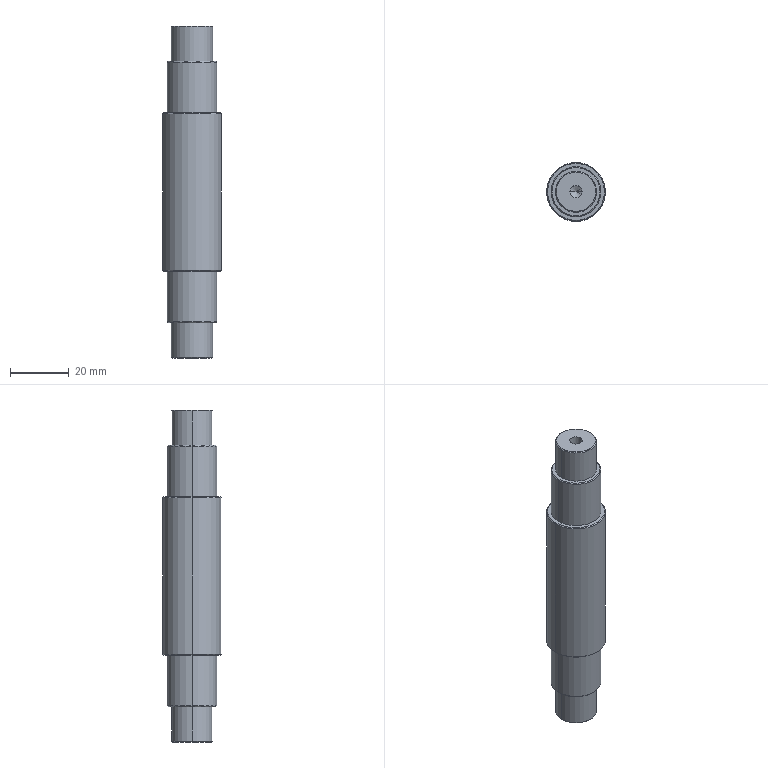Part | NX | features BREP 1 | 1 solid | 36 faces | box 20 x 20 x 113 mm | volume 28190 mm3 | cone 16 | cylinder 14 | plane 6 | commonest cylinder face diameters 4.2 x4 14 x4 17 x4 20 x2
STEP:
#1=CARTESIAN_POINT('',(6.7,0.,56.5));
#2=VERTEX_POINT('',#1);
#3=CARTESIAN_POINT('',(-6.7,0.,56.5));
#4=VERTEX_POINT('',#3);
#5=CARTESIAN_POINT('',(0.,0.,56.5));
#6=DIRECTION('',(0.,0.,1.));
#7=DIRECTION('',(1.,0.,0.));
#8=AXIS2_PLACEMENT_3D('',#5,#6,#7);
#9=CIRCLE('',#8,6.7);
#10=EDGE_CURVE('',#2,#4,#9,.T.);
#11=ORIENTED_EDGE('',*,*,#10,.F.);
#12=CARTESIAN_POINT('',(7.,0.,56.2));
#13=VERTEX_POINT('',#12);
#14=CARTESIAN_POINT('',(6.7,0.,56.5));
#15=DIRECTION('',(0.7071,0.,-0.7071));
#16=VECTOR('',#15,1000.);
#17=LINE('',#14,#16);
#18=EDGE_CURVE('',#2,#13,#17,.T.);
#19=ORIENTED_EDGE('',*,*,#18,.T.);
#20=CARTESIAN_POINT('',(-7.,0.,56.2));
#21=VERTEX_POINT('',#20);
#22=CARTESIAN_POINT('',(0.,0.,56.2));
#23=DIRECTION('',(0.,0.,-1.));
#24=DIRECTION('',(1.,0.,0.));
#25=AXIS2_PLACEMENT_3D('',#22,#23,#24);
#26=CIRCLE('',#25,7.);
#27=EDGE_CURVE('',#21,#13,#26,.T.);
#28=ORIENTED_EDGE('',*,*,#27,.F.);
#29=CARTESIAN_POINT('',(-6.7,0.,56.5));
#30=DIRECTION('',(-0.7071,0.,-0.7071));
#31=VECTOR('',#30,1000.);
#32=LINE('',#29,#31);
#33=EDGE_CURVE('',#4,#21,#32,.T.);
#34=ORIENTED_EDGE('',*,*,#33,.F.);
#35=EDGE_LOOP('',(#11,#19,#28,#34));
#36=FACE_BOUND('',#35,.T.);
#37=CARTESIAN_POINT('',(0.,0.,56.5));
#38=DIRECTION('',(0.,0.,-1.));
#39=DIRECTION('',(-1.,0.,0.));
#40=AXIS2_PLACEMENT_3D('',#37,#38,#39);
#41=CONICAL_SURFACE('',#40,6.7,0.7854);
#42=ADVANCED_FACE('',(#36),#41,.T.);
#43=CARTESIAN_POINT('',(8.2,0.,44.5));
#44=VERTEX_POINT('',#43);
#45=CARTESIAN_POINT('',(-8.2,0.,44.5));
#46=VERTEX_POINT('',#45);
#47=CARTESIAN_POINT('',(0.,0.,44.5));
#48=DIRECTION('',(0.,0.,1.));
#49=DIRECTION('',(1.,0.,0.));
#50=AXIS2_PLACEMENT_3D('',#47,#48,#49);
#51=CIRCLE('',#50,8.2);
#52=EDGE_CURVE('',#44,#46,#51,.T.);
#53=ORIENTED_EDGE('',*,*,#52,.F.);
#54=CARTESIAN_POINT('',(8.5,0.,44.2));
#55=VERTEX_POINT('',#54);
#56=CARTESIAN_POINT('',(8.2,0.,44.5));
#57=DIRECTION('',(0.7071,0.,-0.7071));
#58=VECTOR('',#57,1000.);
#59=LINE('',#56,#58);
#60=EDGE_CURVE('',#44,#55,#59,.T.);
#61=ORIENTED_EDGE('',*,*,#60,.T.);
#62=CARTESIAN_POINT('',(-8.5,0.,44.2));
#63=VERTEX_POINT('',#62);
#64=CARTESIAN_POINT('',(0.,0.,44.2));
#65=DIRECTION('',(0.,0.,-1.));
#66=DIRECTION('',(1.,0.,0.));
#67=AXIS2_PLACEMENT_3D('',#64,#65,#66);
#68=CIRCLE('',#67,8.5);
#69=EDGE_CURVE('',#63,#55,#68,.T.);
#70=ORIENTED_EDGE('',*,*,#69,.F.);
#71=CARTESIAN_POINT('',(-8.2,0.,44.5));
#72=DIRECTION('',(-0.7071,0.,-0.7071));
#73=VECTOR('',#72,1000.);
#74=LINE('',#71,#73);
#75=EDGE_CURVE('',#46,#63,#74,.T.);
#76=ORIENTED_EDGE('',*,*,#75,.F.);
#77=EDGE_LOOP('',(#53,#61,#70,#76));
#78=FACE_BOUND('',#77,.T.);
#79=CARTESIAN_POINT('',(0.,0.,44.5));
#80=DIRECTION('',(0.,0.,-1.));
#81=DIRECTION('',(-1.,0.,0.));
#82=AXIS2_PLACEMENT_3D('',#79,#80,#81);
#83=CONICAL_SURFACE('',#82,8.2,0.7854);
#84=ADVANCED_FACE('',(#78),#83,.T.);
#85=CARTESIAN_POINT('',(9.7,0.,27.));
#86=VERTEX_POINT('',#85);
#87=CARTESIAN_POINT('',(-9.7,0.,27.));
#88=VERTEX_POINT('',#87);
#89=CARTESIAN_POINT('',(0.,0.,27.));
#90=DIRECTION('',(0.,0.,1.));
#91=DIRECTION('',(1.,0.,0.));
#92=AXIS2_PLACEMENT_3D('',#89,#90,#91);
#93=CIRCLE('',#92,9.7);
#94=EDGE_CURVE('',#86,#88,#93,.T.);
#95=ORIENTED_EDGE('',*,*,#94,.F.);
#96=CARTESIAN_POINT('',(10.,0.,26.7));
#97=VERTEX_POINT('',#96);
#98=CARTESIAN_POINT('',(10.,0.,26.7));
#99=DIRECTION('',(0.7071,0.,-0.7071));
#100=VECTOR('',#99,1000.);
#101=LINE('',#98,#100);
#102=EDGE_CURVE('',#86,#97,#101,.T.);
#103=ORIENTED_EDGE('',*,*,#102,.T.);
#104=CARTESIAN_POINT('',(-10.,0.,26.7));
#105=VERTEX_POINT('',#104);
#106=CARTESIAN_POINT('',(0.,0.,26.7));
#107=DIRECTION('',(0.,0.,-1.));
#108=DIRECTION('',(1.,0.,0.));
#109=AXIS2_PLACEMENT_3D('',#106,#107,#108);
#110=CIRCLE('',#109,10.);
#111=EDGE_CURVE('',#105,#97,#110,.T.);
#112=ORIENTED_EDGE('',*,*,#111,.F.);
#113=CARTESIAN_POINT('',(-10.,0.,26.7));
#114=DIRECTION('',(-0.7071,0.,-0.7071));
#115=VECTOR('',#114,1000.);
#116=LINE('',#113,#115);
#117=EDGE_CURVE('',#88,#105,#116,.T.);
#118=ORIENTED_EDGE('',*,*,#117,.F.);
#119=EDGE_LOOP('',(#95,#103,#112,#118));
#120=FACE_BOUND('',#119,.T.);
#121=CARTESIAN_POINT('',(0.,0.,26.7));
#122=DIRECTION('',(0.,0.,-1.));
#123=DIRECTION('',(-1.,0.,0.));
#124=AXIS2_PLACEMENT_3D('',#121,#122,#123);
#125=CONICAL_SURFACE('',#124,10.,0.7854);
#126=ADVANCED_FACE('',(#120),#125,.T.);
#127=CARTESIAN_POINT('',(-9.7,0.,-27.));
#128=VERTEX_POINT('',#127);
#129=CARTESIAN_POINT('',(9.7,0.,-27.));
#130=VERTEX_POINT('',#129);
#131=CARTESIAN_POINT('',(0.,0.,-27.));
#132=DIRECTION('',(0.,0.,-1.));
#133=DIRECTION('',(-1.,0.,0.));
#134=AXIS2_PLACEMENT_3D('',#131,#132,#133);
#135=CIRCLE('',#134,9.7);
#136=EDGE_CURVE('',#128,#130,#135,.T.);
#137=ORIENTED_EDGE('',*,*,#136,.F.);
#138=CARTESIAN_POINT('',(-10.,0.,-26.7));
#139=VERTEX_POINT('',#138);
#140=CARTESIAN_POINT('',(-9.7,0.,-27.));
#141=DIRECTION('',(-0.7071,0.,0.7071));
#142=VECTOR('',#141,1000.);
#143=LINE('',#140,#142);
#144=EDGE_CURVE('',#139,#128,#143,.F.);
#145=ORIENTED_EDGE('',*,*,#144,.F.);
#146=CARTESIAN_POINT('',(10.,0.,-26.7));
#147=VERTEX_POINT('',#146);
#148=CARTESIAN_POINT('',(0.,0.,-26.7));
#149=DIRECTION('',(0.,0.,1.));
#150=DIRECTION('',(-1.,0.,0.));
#151=AXIS2_PLACEMENT_3D('',#148,#149,#150);
#152=CIRCLE('',#151,10.);
#153=EDGE_CURVE('',#147,#139,#152,.T.);
#154=ORIENTED_EDGE('',*,*,#153,.F.);
#155=CARTESIAN_POINT('',(9.7,0.,-27.));
#156=DIRECTION('',(0.7071,0.,0.7071));
#157=VECTOR('',#156,1000.);
#158=LINE('',#155,#157);
#159=EDGE_CURVE('',#147,#130,#158,.F.);
#160=ORIENTED_EDGE('',*,*,#159,.T.);
#161=EDGE_LOOP('',(#137,#145,#154,#160));
#162=FACE_BOUND('',#161,.T.);
#163=CARTESIAN_POINT('',(0.,0.,-27.));
#164=DIRECTION('',(0.,0.,1.));
#165=DIRECTION('',(1.,0.,0.));
#166=AXIS2_PLACEMENT_3D('',#163,#164,#165);
#167=CONICAL_SURFACE('',#166,9.7,0.7854);
#168=ADVANCED_FACE('',(#162),#167,.T.);
#169=CARTESIAN_POINT('',(-8.2,0.,-44.5));
#170=VERTEX_POINT('',#169);
#171=CARTESIAN_POINT('',(8.2,0.,-44.5));
#172=VERTEX_POINT('',#171);
#173=CARTESIAN_POINT('',(0.,0.,-44.5));
#174=DIRECTION('',(0.,0.,-1.));
#175=DIRECTION('',(1.,0.,0.));
#176=AXIS2_PLACEMENT_3D('',#173,#174,#175);
#177=CIRCLE('',#176,8.2);
#178=EDGE_CURVE('',#170,#172,#177,.T.);
#179=ORIENTED_EDGE('',*,*,#178,.F.);
#180=CARTESIAN_POINT('',(-8.5,0.,-44.2));
#181=VERTEX_POINT('',#180);
#182=CARTESIAN_POINT('',(-8.5,0.,-44.2));
#183=DIRECTION('',(-0.7071,0.,0.7071));
#184=VECTOR('',#183,1000.);
#185=LINE('',#182,#184);
#186=EDGE_CURVE('',#181,#170,#185,.F.);
#187=ORIENTED_EDGE('',*,*,#186,.F.);
#188=CARTESIAN_POINT('',(8.5,0.,-44.2));
#189=VERTEX_POINT('',#188);
#190=CARTESIAN_POINT('',(0.,0.,-44.2));
#191=DIRECTION('',(0.,0.,1.));
#192=DIRECTION('',(1.,0.,0.));
#193=AXIS2_PLACEMENT_3D('',#190,#191,#192);
#194=CIRCLE('',#193,8.5);
#195=EDGE_CURVE('',#189,#181,#194,.T.);
#196=ORIENTED_EDGE('',*,*,#195,.F.);
#197=CARTESIAN_POINT('',(8.5,0.,-44.2));
#198=DIRECTION('',(0.7071,0.,0.7071));
#199=VECTOR('',#198,1000.);
#200=LINE('',#197,#199);
#201=EDGE_CURVE('',#189,#172,#200,.F.);
#202=ORIENTED_EDGE('',*,*,#201,.T.);
#203=EDGE_LOOP('',(#179,#187,#196,#202));
#204=FACE_BOUND('',#203,.T.);
#205=CARTESIAN_POINT('',(0.,0.,-44.2));
#206=DIRECTION('',(0.,0.,1.));
#207=DIRECTION('',(1.,0.,0.));
#208=AXIS2_PLACEMENT_3D('',#205,#206,#207);
#209=CONICAL_SURFACE('',#208,8.5,0.7854);
#210=ADVANCED_FACE('',(#204),#209,.T.);
#211=CARTESIAN_POINT('',(-6.7,0.,-56.5));
#212=VERTEX_POINT('',#211);
#213=CARTESIAN_POINT('',(6.7,0.,-56.5));
#214=VERTEX_POINT('',#213);
#215=CARTESIAN_POINT('',(0.,0.,-56.5));
#216=DIRECTION('',(0.,0.,-1.));
#217=DIRECTION('',(-1.,0.,0.));
#218=AXIS2_PLACEMENT_3D('',#215,#216,#217);
#219=CIRCLE('',#218,6.7);
#220=EDGE_CURVE('',#212,#214,#219,.T.);
#221=ORIENTED_EDGE('',*,*,#220,.F.);
#222=CARTESIAN_POINT('',(-7.,0.,-56.2));
#223=VERTEX_POINT('',#222);
#224=CARTESIAN_POINT('',(-6.7,0.,-56.5));
#225=DIRECTION('',(-0.7071,0.,0.7071));
#226=VECTOR('',#225,1000.);
#227=LINE('',#224,#226);
#228=EDGE_CURVE('',#223,#212,#227,.F.);
#229=ORIENTED_EDGE('',*,*,#228,.F.);
#230=CARTESIAN_POINT('',(7.,0.,-56.2));
#231=VERTEX_POINT('',#230);
#232=CARTESIAN_POINT('',(0.,0.,-56.2));
#233=DIRECTION('',(0.,0.,1.));
#234=DIRECTION('',(-1.,0.,0.));
#235=AXIS2_PLACEMENT_3D('',#232,#233,#234);
#236=CIRCLE('',#235,7.);
#237=EDGE_CURVE('',#231,#223,#236,.T.);
#238=ORIENTED_EDGE('',*,*,#237,.F.);
#239=CARTESIAN_POINT('',(6.7,0.,-56.5));
#240=DIRECTION('',(0.7071,0.,0.7071));
#241=VECTOR('',#240,1000.);
#242=LINE('',#239,#241);
#243=EDGE_CURVE('',#231,#214,#242,.F.);
#244=ORIENTED_EDGE('',*,*,#243,.T.);
#245=EDGE_LOOP('',(#221,#229,#238,#244));
#246=FACE_BOUND('',#245,.T.);
#247=CARTESIAN_POINT('',(0.,0.,-56.5));
#248=DIRECTION('',(0.,0.,1.));
#249=DIRECTION('',(1.,0.,0.));
#250=AXIS2_PLACEMENT_3D('',#247,#248,#249);
#251=CONICAL_SURFACE('',#250,6.7,0.7854);
#252=ADVANCED_FACE('',(#246),#251,.T.);
#253=CARTESIAN_POINT('',(-8.5,0.,-27.));
#254=VERTEX_POINT('',#253);
#255=CARTESIAN_POINT('',(8.5,0.,-27.));
#256=VERTEX_POINT('',#255);
#257=CARTESIAN_POINT('',(0.,0.,-27.));
#258=DIRECTION('',(0.,0.,-1.));
#259=DIRECTION('',(-1.,0.,0.));
#260=AXIS2_PLACEMENT_3D('',#257,#258,#259);
#261=CIRCLE('',#260,8.5);
#262=EDGE_CURVE('',#254,#256,#261,.T.);
#263=ORIENTED_EDGE('',*,*,#262,.T.);
#264=CARTESIAN_POINT('',(8.5,0.,44.5));
#265=DIRECTION('',(0.,0.,-1.));
#266=VECTOR('',#265,1000.);
#267=LINE('',#264,#266);
#268=EDGE_CURVE('',#256,#189,#267,.T.);
#269=ORIENTED_EDGE('',*,*,#268,.T.);
#270=ORIENTED_EDGE('',*,*,#195,.T.);
#271=CARTESIAN_POINT('',(-8.5,0.,44.5));
#272=DIRECTION('',(0.,0.,-1.));
#273=VECTOR('',#272,1000.);
#274=LINE('',#271,#273);
#275=EDGE_CURVE('',#254,#181,#274,.T.);
#276=ORIENTED_EDGE('',*,*,#275,.F.);
#277=EDGE_LOOP('',(#263,#269,#270,#276));
#278=FACE_BOUND('',#277,.T.);
#279=CARTESIAN_POINT('',(0.,0.,44.5));
#280=DIRECTION('',(0.,0.,-1.));
#281=DIRECTION('',(-1.,0.,0.));
#282=AXIS2_PLACEMENT_3D('',#279,#280,#281);
#283=CYLINDRICAL_SURFACE('',#282,8.5);
#284=ADVANCED_FACE('',(#278),#283,.T.);
#285=ORIENTED_EDGE('',*,*,#237,.T.);
#286=CARTESIAN_POINT('',(-7.,0.,-44.5));
#287=VERTEX_POINT('',#286);
#288=CARTESIAN_POINT('',(-7.,0.,-56.5));
#289=DIRECTION('',(0.,0.,1.));
#290=VECTOR('',#289,1000.);
#291=LINE('',#288,#290);
#292=EDGE_CURVE('',#287,#223,#291,.F.);
#293=ORIENTED_EDGE('',*,*,#292,.F.);
#294=CARTESIAN_POINT('',(7.,0.,-44.5));
#295=VERTEX_POINT('',#294);
#296=CARTESIAN_POINT('',(0.,0.,-44.5));
#297=DIRECTION('',(0.,0.,-1.));
#298=DIRECTION('',(1.,0.,0.));
#299=AXIS2_PLACEMENT_3D('',#296,#297,#298);
#300=CIRCLE('',#299,7.);
#301=EDGE_CURVE('',#287,#295,#300,.T.);
#302=ORIENTED_EDGE('',*,*,#301,.T.);
#303=CARTESIAN_POINT('',(7.,0.,-56.5));
#304=DIRECTION('',(0.,0.,1.));
#305=VECTOR('',#304,1000.);
#306=LINE('',#303,#305);
#307=EDGE_CURVE('',#295,#231,#306,.F.);
#308=ORIENTED_EDGE('',*,*,#307,.T.);
#309=EDGE_LOOP('',(#285,#293,#302,#308));
#310=FACE_BOUND('',#309,.T.);
#311=CARTESIAN_POINT('',(0.,0.,-56.5));
#312=DIRECTION('',(0.,0.,1.));
#313=DIRECTION('',(1.,0.,0.));
#314=AXIS2_PLACEMENT_3D('',#311,#312,#313);
#315=CYLINDRICAL_SURFACE('',#314,7.);
#316=ADVANCED_FACE('',(#310),#315,.T.);
#317=CARTESIAN_POINT('',(2.1,0.,-42.5));
#318=VERTEX_POINT('',#317);
#319=CARTESIAN_POINT('',(-2.1,0.,-42.5));
#320=VERTEX_POINT('',#319);
#321=CARTESIAN_POINT('',(0.,0.,-42.5));
#322=DIRECTION('',(0.,0.,-1.));
#323=DIRECTION('',(-1.,0.,0.));
#324=AXIS2_PLACEMENT_3D('',#321,#322,#323);
#325=CIRCLE('',#324,2.1);
#326=EDGE_CURVE('',#318,#320,#325,.T.);
#327=ORIENTED_EDGE('',*,*,#326,.F.);
#328=CARTESIAN_POINT('',(2.1,0.,-56.5));
#329=VERTEX_POINT('',#328);
#330=CARTESIAN_POINT('',(2.1,0.,-56.5));
#331=DIRECTION('',(0.,0.,-1.));
#332=VECTOR('',#331,1000.);
#333=LINE('',#330,#332);
#334=EDGE_CURVE('',#318,#329,#333,.T.);
#335=ORIENTED_EDGE('',*,*,#334,.T.);
#336=CARTESIAN_POINT('',(-2.1,0.,-56.5));
#337=VERTEX_POINT('',#336);
#338=CARTESIAN_POINT('',(0.,0.,-56.5));
#339=DIRECTION('',(0.,0.,-1.));
#340=DIRECTION('',(-1.,0.,0.));
#341=AXIS2_PLACEMENT_3D('',#338,#339,#340);
#342=CIRCLE('',#341,2.1);
#343=EDGE_CURVE('',#329,#337,#342,.T.);
#344=ORIENTED_EDGE('',*,*,#343,.T.);
#345=CARTESIAN_POINT('',(-2.1,0.,-56.5));
#346=DIRECTION('',(0.,0.,-1.));
#347=VECTOR('',#346,1000.);
#348=LINE('',#345,#347);
#349=EDGE_CURVE('',#320,#337,#348,.T.);
#350=ORIENTED_EDGE('',*,*,#349,.F.);
#351=EDGE_LOOP('',(#327,#335,#344,#350));
#352=FACE_BOUND('',#351,.T.);
#353=CARTESIAN_POINT('',(0.,0.,-56.5));
#354=DIRECTION('',(0.,0.,-1.));
#355=DIRECTION('',(-1.,0.,0.));
#356=AXIS2_PLACEMENT_3D('',#353,#354,#355);
#357=CYLINDRICAL_SURFACE('',#356,2.1);
#358=ADVANCED_FACE('',(#352),#357,.F.);
#359=CARTESIAN_POINT('',(0.,0.,-41.238));
#360=VERTEX_POINT('',#359);
#361=CARTESIAN_POINT('',(-2.1,0.,-42.5));
#362=DIRECTION('',(-0.8572,0.,-0.515));
#363=VECTOR('',#362,1000.);
#364=LINE('',#361,#363);
#365=EDGE_CURVE('',#360,#320,#364,.T.);
#366=ORIENTED_EDGE('',*,*,#365,.F.);
#367=CARTESIAN_POINT('',(2.1,0.,-42.5));
#368=DIRECTION('',(0.8572,0.,-0.515));
#369=VECTOR('',#368,1000.);
#370=LINE('',#367,#369);
#371=EDGE_CURVE('',#360,#318,#370,.T.);
#372=ORIENTED_EDGE('',*,*,#371,.T.);
#373=ORIENTED_EDGE('',*,*,#326,.T.);
#374=EDGE_LOOP('',(#366,#372,#373));
#375=FACE_BOUND('',#374,.T.);
#376=CARTESIAN_POINT('',(0.,0.,-42.5));
#377=DIRECTION('',(0.,0.,-1.));
#378=DIRECTION('',(-1.,0.,0.));
#379=AXIS2_PLACEMENT_3D('',#376,#377,#378);
#380=CONICAL_SURFACE('',#379,2.1,1.03);
#381=ADVANCED_FACE('',(#375),#380,.F.);
#382=ORIENTED_EDGE('',*,*,#111,.T.);
#383=CARTESIAN_POINT('',(10.,0.,27.));
#384=DIRECTION('',(0.,0.,-1.));
#385=VECTOR('',#384,1000.);
#386=LINE('',#383,#385);
#387=EDGE_CURVE('',#97,#147,#386,.T.);
#388=ORIENTED_EDGE('',*,*,#387,.T.);
#389=ORIENTED_EDGE('',*,*,#153,.T.);
#390=CARTESIAN_POINT('',(-10.,0.,27.));
#391=DIRECTION('',(0.,0.,-1.));
#392=VECTOR('',#391,1000.);
#393=LINE('',#390,#392);
#394=EDGE_CURVE('',#105,#139,#393,.T.);
#395=ORIENTED_EDGE('',*,*,#394,.F.);
#396=EDGE_LOOP('',(#382,#388,#389,#395));
#397=FACE_BOUND('',#396,.T.);
#398=CARTESIAN_POINT('',(0.,0.,27.));
#399=DIRECTION('',(0.,0.,-1.));
#400=DIRECTION('',(-1.,0.,0.));
#401=AXIS2_PLACEMENT_3D('',#398,#399,#400);
#402=CYLINDRICAL_SURFACE('',#401,10.);
#403=ADVANCED_FACE('',(#397),#402,.T.);
#404=CARTESIAN_POINT('',(-2.1,0.,42.5));
#405=VERTEX_POINT('',#404);
#406=CARTESIAN_POINT('',(2.1,0.,42.5));
#407=VERTEX_POINT('',#406);
#408=CARTESIAN_POINT('',(0.,0.,42.5));
#409=DIRECTION('',(0.,0.,1.));
#410=DIRECTION('',(1.,0.,0.));
#411=AXIS2_PLACEMENT_3D('',#408,#409,#410);
#412=CIRCLE('',#411,2.1);
#413=EDGE_CURVE('',#405,#407,#412,.T.);
#414=ORIENTED_EDGE('',*,*,#413,.F.);
#415=CARTESIAN_POINT('',(-2.1,0.,56.5));
#416=VERTEX_POINT('',#415);
#417=CARTESIAN_POINT('',(-2.1,0.,56.5));
#418=DIRECTION('',(0.,0.,1.));
#419=VECTOR('',#418,1000.);
#420=LINE('',#417,#419);
#421=EDGE_CURVE('',#416,#405,#420,.F.);
#422=ORIENTED_EDGE('',*,*,#421,.F.);
#423=CARTESIAN_POINT('',(2.1,0.,56.5));
#424=VERTEX_POINT('',#423);
#425=CARTESIAN_POINT('',(0.,0.,56.5));
#426=DIRECTION('',(0.,0.,1.));
#427=DIRECTION('',(1.,0.,0.));
#428=AXIS2_PLACEMENT_3D('',#425,#426,#427);
#429=CIRCLE('',#428,2.1);
#430=EDGE_CURVE('',#416,#424,#429,.T.);
#431=ORIENTED_EDGE('',*,*,#430,.T.);
#432=CARTESIAN_POINT('',(2.1,0.,56.5));
#433=DIRECTION('',(0.,0.,1.));
#434=VECTOR('',#433,1000.);
#435=LINE('',#432,#434);
#436=EDGE_CURVE('',#424,#407,#435,.F.);
#437=ORIENTED_EDGE('',*,*,#436,.T.);
#438=EDGE_LOOP('',(#414,#422,#431,#437));
#439=FACE_BOUND('',#438,.T.);
#440=CARTESIAN_POINT('',(0.,0.,56.5));
#441=DIRECTION('',(0.,0.,1.));
#442=DIRECTION('',(1.,0.,0.));
#443=AXIS2_PLACEMENT_3D('',#440,#441,#442);
#444=CYLINDRICAL_SURFACE('',#443,2.1);
#445=ADVANCED_FACE('',(#439),#444,.F.);
#446=CARTESIAN_POINT('',(0.,0.,41.238));
#447=VERTEX_POINT('',#446);
#448=CARTESIAN_POINT('',(2.1,0.,42.5));
#449=DIRECTION('',(0.8572,0.,0.515));
#450=VECTOR('',#449,1000.);
#451=LINE('',#448,#450);
#452=EDGE_CURVE('',#407,#447,#451,.F.);
#453=ORIENTED_EDGE('',*,*,#452,.T.);
#454=CARTESIAN_POINT('',(-2.1,0.,42.5));
#455=DIRECTION('',(-0.8572,0.,0.515));
#456=VECTOR('',#455,1000.);
#457=LINE('',#454,#456);
#458=EDGE_CURVE('',#405,#447,#457,.F.);
#459=ORIENTED_EDGE('',*,*,#458,.F.);
#460=ORIENTED_EDGE('',*,*,#413,.T.);
#461=EDGE_LOOP('',(#453,#459,#460));
#462=FACE_BOUND('',#461,.T.);
#463=CARTESIAN_POINT('',(0.,0.,42.5));
#464=DIRECTION('',(0.,0.,1.));
#465=DIRECTION('',(1.,0.,0.));
#466=AXIS2_PLACEMENT_3D('',#463,#464,#465);
#467=CONICAL_SURFACE('',#466,2.1,1.03);
#468=ADVANCED_FACE('',(#462),#467,.F.);
#469=ORIENTED_EDGE('',*,*,#27,.T.);
#470=CARTESIAN_POINT('',(7.,0.,44.5));
#471=VERTEX_POINT('',#470);
#472=CARTESIAN_POINT('',(7.,0.,56.5));
#473=DIRECTION('',(0.,0.,-1.));
#474=VECTOR('',#473,1000.);
#475=LINE('',#472,#474);
#476=EDGE_CURVE('',#13,#471,#475,.T.);
#477=ORIENTED_EDGE('',*,*,#476,.T.);
#478=CARTESIAN_POINT('',(-7.,0.,44.5));
#479=VERTEX_POINT('',#478);
#480=CARTESIAN_POINT('',(0.,0.,44.5));
#481=DIRECTION('',(0.,0.,1.));
#482=DIRECTION('',(1.,0.,0.));
#483=AXIS2_PLACEMENT_3D('',#480,#481,#482);
#484=CIRCLE('',#483,7.);
#485=EDGE_CURVE('',#471,#479,#484,.T.);
#486=ORIENTED_EDGE('',*,*,#485,.T.);
#487=CARTESIAN_POINT('',(-7.,0.,56.5));
#488=DIRECTION('',(0.,0.,-1.));
#489=VECTOR('',#488,1000.);
#490=LINE('',#487,#489);
#491=EDGE_CURVE('',#21,#479,#490,.T.);
#492=ORIENTED_EDGE('',*,*,#491,.F.);
#493=EDGE_LOOP('',(#469,#477,#486,#492));
#494=FACE_BOUND('',#493,.T.);
#495=CARTESIAN_POINT('',(0.,0.,56.5));
#496=DIRECTION('',(0.,0.,-1.));
#497=DIRECTION('',(-1.,0.,0.));
#498=AXIS2_PLACEMENT_3D('',#495,#496,#497);
#499=CYLINDRICAL_SURFACE('',#498,7.);
#500=ADVANCED_FACE('',(#494),#499,.T.);
#501=ORIENTED_EDGE('',*,*,#69,.T.);
#502=CARTESIAN_POINT('',(8.5,0.,27.));
#503=VERTEX_POINT('',#502);
#504=CARTESIAN_POINT('',(8.5,0.,44.5));
#505=DIRECTION('',(0.,0.,-1.));
#506=VECTOR('',#505,1000.);
#507=LINE('',#504,#506);
#508=EDGE_CURVE('',#55,#503,#507,.T.);
#509=ORIENTED_EDGE('',*,*,#508,.T.);
#510=CARTESIAN_POINT('',(-8.5,0.,27.));
#511=VERTEX_POINT('',#510);
#512=CARTESIAN_POINT('',(0.,0.,27.));
#513=DIRECTION('',(0.,0.,1.));
#514=DIRECTION('',(1.,0.,0.));
#515=AXIS2_PLACEMENT_3D('',#512,#513,#514);
#516=CIRCLE('',#515,8.5);
#517=EDGE_CURVE('',#503,#511,#516,.T.);
#518=ORIENTED_EDGE('',*,*,#517,.T.);
#519=CARTESIAN_POINT('',(-8.5,0.,44.5));
#520=DIRECTION('',(0.,0.,-1.));
#521=VECTOR('',#520,1000.);
#522=LINE('',#519,#521);
#523=EDGE_CURVE('',#63,#511,#522,.T.);
#524=ORIENTED_EDGE('',*,*,#523,.F.);
#525=EDGE_LOOP('',(#501,#509,#518,#524));
#526=FACE_BOUND('',#525,.T.);
#527=CARTESIAN_POINT('',(0.,0.,44.5));
#528=DIRECTION('',(0.,0.,-1.));
#529=DIRECTION('',(-1.,0.,0.));
#530=AXIS2_PLACEMENT_3D('',#527,#528,#529);
#531=CYLINDRICAL_SURFACE('',#530,8.5);
#532=ADVANCED_FACE('',(#526),#531,.T.);
#533=ORIENTED_EDGE('',*,*,#508,.F.);
#534=CARTESIAN_POINT('',(0.,0.,44.2));
#535=DIRECTION('',(0.,0.,-1.));
#536=DIRECTION('',(1.,0.,0.));
#537=AXIS2_PLACEMENT_3D('',#534,#535,#536);
#538=CIRCLE('',#537,8.5);
#539=EDGE_CURVE('',#55,#63,#538,.T.);
#540=ORIENTED_EDGE('',*,*,#539,.T.);
#541=ORIENTED_EDGE('',*,*,#523,.T.);
#542=CARTESIAN_POINT('',(0.,0.,27.));
#543=DIRECTION('',(0.,0.,1.));
#544=DIRECTION('',(1.,0.,0.));
#545=AXIS2_PLACEMENT_3D('',#542,#543,#544);
#546=CIRCLE('',#545,8.5);
#547=EDGE_CURVE('',#511,#503,#546,.T.);
#548=ORIENTED_EDGE('',*,*,#547,.T.);
#549=EDGE_LOOP('',(#533,#540,#541,#548));
#550=FACE_BOUND('',#549,.T.);
#551=CARTESIAN_POINT('',(0.,0.,44.5));
#552=DIRECTION('',(0.,0.,-1.));
#553=DIRECTION('',(-1.,0.,0.));
#554=AXIS2_PLACEMENT_3D('',#551,#552,#553);
#555=CYLINDRICAL_SURFACE('',#554,8.5);
#556=ADVANCED_FACE('',(#550),#555,.T.);
#557=CARTESIAN_POINT('',(0.,0.,44.5));
#558=DIRECTION('',(0.,0.,1.));
#559=DIRECTION('',(1.,0.,0.));
#560=AXIS2_PLACEMENT_3D('',#557,#558,#559);
#561=CIRCLE('',#560,8.2);
#562=EDGE_CURVE('',#46,#44,#561,.T.);
#563=ORIENTED_EDGE('',*,*,#562,.T.);
#564=ORIENTED_EDGE('',*,*,#52,.T.);
#565=EDGE_LOOP('',(#563,#564));
#566=FACE_BOUND('',#565,.T.);
#567=CARTESIAN_POINT('',(0.,0.,44.5));
#568=DIRECTION('',(0.,0.,1.));
#569=DIRECTION('',(1.,0.,0.));
#570=AXIS2_PLACEMENT_3D('',#567,#568,#569);
#571=CIRCLE('',#570,7.);
#572=EDGE_CURVE('',#479,#471,#571,.T.);
#573=ORIENTED_EDGE('',*,*,#572,.F.);
#574=ORIENTED_EDGE('',*,*,#485,.F.);
#575=EDGE_LOOP('',(#573,#574));
#576=FACE_BOUND('',#575,.T.);
#577=CARTESIAN_POINT('',(0.,0.,44.5));
#578=DIRECTION('',(0.,0.,1.));
#579=DIRECTION('',(1.,0.,0.));
#580=AXIS2_PLACEMENT_3D('',#577,#578,#579);
#581=PLANE('',#580);
#582=ADVANCED_FACE('',(#566,#576),#581,.T.);
#583=ORIENTED_EDGE('',*,*,#476,.F.);
#584=CARTESIAN_POINT('',(0.,0.,56.2));
#585=DIRECTION('',(0.,0.,-1.));
#586=DIRECTION('',(1.,0.,0.));
#587=AXIS2_PLACEMENT_3D('',#584,#585,#586);
#588=CIRCLE('',#587,7.);
#589=EDGE_CURVE('',#13,#21,#588,.T.);
#590=ORIENTED_EDGE('',*,*,#589,.T.);
#591=ORIENTED_EDGE('',*,*,#491,.T.);
#592=ORIENTED_EDGE('',*,*,#572,.T.);
#593=EDGE_LOOP('',(#583,#590,#591,#592));
#594=FACE_BOUND('',#593,.T.);
#595=CARTESIAN_POINT('',(0.,0.,56.5));
#596=DIRECTION('',(0.,0.,-1.));
#597=DIRECTION('',(-1.,0.,0.));
#598=AXIS2_PLACEMENT_3D('',#595,#596,#597);
#599=CYLINDRICAL_SURFACE('',#598,7.);
#600=ADVANCED_FACE('',(#594),#599,.T.);
#601=CARTESIAN_POINT('',(0.,0.,56.5));
#602=DIRECTION('',(0.,0.,1.));
#603=DIRECTION('',(1.,0.,0.));
#604=AXIS2_PLACEMENT_3D('',#601,#602,#603);
#605=CIRCLE('',#604,6.7);
#606=EDGE_CURVE('',#4,#2,#605,.T.);
#607=ORIENTED_EDGE('',*,*,#606,.T.);
#608=ORIENTED_EDGE('',*,*,#10,.T.);
#609=EDGE_LOOP('',(#607,#608));
#610=FACE_BOUND('',#609,.T.);
#611=CARTESIAN_POINT('',(0.,0.,56.5));
#612=DIRECTION('',(0.,0.,1.));
#613=DIRECTION('',(1.,0.,0.));
#614=AXIS2_PLACEMENT_3D('',#611,#612,#613);
#615=CIRCLE('',#614,2.1);
#616=EDGE_CURVE('',#424,#416,#615,.T.);
#617=ORIENTED_EDGE('',*,*,#616,.F.);
#618=ORIENTED_EDGE('',*,*,#430,.F.);
#619=EDGE_LOOP('',(#617,#618));
#620=FACE_BOUND('',#619,.T.);
#621=CARTESIAN_POINT('',(0.,0.,56.5));
#622=DIRECTION('',(0.,0.,1.));
#623=DIRECTION('',(1.,0.,0.));
#624=AXIS2_PLACEMENT_3D('',#621,#622,#623);
#625=PLANE('',#624);
#626=ADVANCED_FACE('',(#610,#620),#625,.T.);
#627=ORIENTED_EDGE('',*,*,#458,.T.);
#628=ORIENTED_EDGE('',*,*,#452,.F.);
#629=CARTESIAN_POINT('',(0.,0.,42.5));
#630=DIRECTION('',(0.,0.,1.));
#631=DIRECTION('',(1.,0.,0.));
#632=AXIS2_PLACEMENT_3D('',#629,#630,#631);
#633=CIRCLE('',#632,2.1);
#634=EDGE_CURVE('',#407,#405,#633,.T.);
#635=ORIENTED_EDGE('',*,*,#634,.T.);
#636=EDGE_LOOP('',(#627,#628,#635));
#637=FACE_BOUND('',#636,.T.);
#638=CARTESIAN_POINT('',(0.,0.,42.5));
#639=DIRECTION('',(0.,0.,1.));
#640=DIRECTION('',(1.,0.,0.));
#641=AXIS2_PLACEMENT_3D('',#638,#639,#640);
#642=CONICAL_SURFACE('',#641,2.1,1.03);
#643=ADVANCED_FACE('',(#637),#642,.F.);
#644=ORIENTED_EDGE('',*,*,#421,.T.);
#645=ORIENTED_EDGE('',*,*,#634,.F.);
#646=ORIENTED_EDGE('',*,*,#436,.F.);
#647=ORIENTED_EDGE('',*,*,#616,.T.);
#648=EDGE_LOOP('',(#644,#645,#646,#647));
#649=FACE_BOUND('',#648,.T.);
#650=CARTESIAN_POINT('',(0.,0.,56.5));
#651=DIRECTION('',(0.,0.,1.));
#652=DIRECTION('',(1.,0.,0.));
#653=AXIS2_PLACEMENT_3D('',#650,#651,#652);
#654=CYLINDRICAL_SURFACE('',#653,2.1);
#655=ADVANCED_FACE('',(#649),#654,.F.);
#656=CARTESIAN_POINT('',(0.,0.,27.));
#657=DIRECTION('',(0.,0.,1.));
#658=DIRECTION('',(1.,0.,0.));
#659=AXIS2_PLACEMENT_3D('',#656,#657,#658);
#660=CIRCLE('',#659,9.7);
#661=EDGE_CURVE('',#88,#86,#660,.T.);
#662=ORIENTED_EDGE('',*,*,#661,.T.);
#663=ORIENTED_EDGE('',*,*,#94,.T.);
#664=EDGE_LOOP('',(#662,#663));
#665=FACE_BOUND('',#664,.T.);
#666=ORIENTED_EDGE('',*,*,#547,.F.);
#667=ORIENTED_EDGE('',*,*,#517,.F.);
#668=EDGE_LOOP('',(#666,#667));
#669=FACE_BOUND('',#668,.T.);
#670=CARTESIAN_POINT('',(0.,10.,27.));
#671=DIRECTION('',(0.,0.,1.));
#672=DIRECTION('',(1.,0.,0.));
#673=AXIS2_PLACEMENT_3D('',#670,#671,#672);
#674=PLANE('',#673);
#675=ADVANCED_FACE('',(#665,#669),#674,.T.);
#676=CARTESIAN_POINT('',(0.,0.,-27.));
#677=DIRECTION('',(0.,0.,-1.));
#678=DIRECTION('',(-1.,0.,0.));
#679=AXIS2_PLACEMENT_3D('',#676,#677,#678);
#680=CIRCLE('',#679,9.7);
#681=EDGE_CURVE('',#130,#128,#680,.T.);
#682=ORIENTED_EDGE('',*,*,#681,.T.);
#683=ORIENTED_EDGE('',*,*,#136,.T.);
#684=EDGE_LOOP('',(#682,#683));
#685=FACE_BOUND('',#684,.T.);
#686=ORIENTED_EDGE('',*,*,#262,.F.);
#687=CARTESIAN_POINT('',(0.,0.,-27.));
#688=DIRECTION('',(0.,0.,-1.));
#689=DIRECTION('',(-1.,0.,0.));
#690=AXIS2_PLACEMENT_3D('',#687,#688,#689);
#691=CIRCLE('',#690,8.5);
#692=EDGE_CURVE('',#256,#254,#691,.T.);
#693=ORIENTED_EDGE('',*,*,#692,.F.);
#694=EDGE_LOOP('',(#686,#693));
#695=FACE_BOUND('',#694,.T.);
#696=CARTESIAN_POINT('',(0.,0.,-27.));
#697=DIRECTION('',(0.,0.,-1.));
#698=DIRECTION('',(0.,-1.,0.));
#699=AXIS2_PLACEMENT_3D('',#696,#697,#698);
#700=PLANE('',#699);
#701=ADVANCED_FACE('',(#685,#695),#700,.T.);
#702=ORIENTED_EDGE('',*,*,#387,.F.);
#703=CARTESIAN_POINT('',(0.,0.,26.7));
#704=DIRECTION('',(0.,0.,-1.));
#705=DIRECTION('',(1.,0.,0.));
#706=AXIS2_PLACEMENT_3D('',#703,#704,#705);
#707=CIRCLE('',#706,10.);
#708=EDGE_CURVE('',#97,#105,#707,.T.);
#709=ORIENTED_EDGE('',*,*,#708,.T.);
#710=ORIENTED_EDGE('',*,*,#394,.T.);
#711=CARTESIAN_POINT('',(0.,0.,-26.7));
#712=DIRECTION('',(0.,0.,1.));
#713=DIRECTION('',(-1.,0.,0.));
#714=AXIS2_PLACEMENT_3D('',#711,#712,#713);
#715=CIRCLE('',#714,10.);
#716=EDGE_CURVE('',#139,#147,#715,.T.);
#717=ORIENTED_EDGE('',*,*,#716,.T.);
#718=EDGE_LOOP('',(#702,#709,#710,#717));
#719=FACE_BOUND('',#718,.T.);
#720=CARTESIAN_POINT('',(0.,0.,27.));
#721=DIRECTION('',(0.,0.,-1.));
#722=DIRECTION('',(-1.,0.,0.));
#723=AXIS2_PLACEMENT_3D('',#720,#721,#722);
#724=CYLINDRICAL_SURFACE('',#723,10.);
#725=ADVANCED_FACE('',(#719),#724,.T.);
#726=ORIENTED_EDGE('',*,*,#371,.F.);
#727=ORIENTED_EDGE('',*,*,#365,.T.);
#728=CARTESIAN_POINT('',(0.,0.,-42.5));
#729=DIRECTION('',(0.,0.,-1.));
#730=DIRECTION('',(-1.,0.,0.));
#731=AXIS2_PLACEMENT_3D('',#728,#729,#730);
#732=CIRCLE('',#731,2.1);
#733=EDGE_CURVE('',#320,#318,#732,.T.);
#734=ORIENTED_EDGE('',*,*,#733,.T.);
#735=EDGE_LOOP('',(#726,#727,#734));
#736=FACE_BOUND('',#735,.T.);
#737=CARTESIAN_POINT('',(0.,0.,-42.5));
#738=DIRECTION('',(0.,0.,-1.));
#739=DIRECTION('',(-1.,0.,0.));
#740=AXIS2_PLACEMENT_3D('',#737,#738,#739);
#741=CONICAL_SURFACE('',#740,2.1,1.03);
#742=ADVANCED_FACE('',(#736),#741,.F.);
#743=ORIENTED_EDGE('',*,*,#334,.F.);
#744=ORIENTED_EDGE('',*,*,#733,.F.);
#745=ORIENTED_EDGE('',*,*,#349,.T.);
#746=CARTESIAN_POINT('',(0.,0.,-56.5));
#747=DIRECTION('',(0.,0.,-1.));
#748=DIRECTION('',(-1.,0.,0.));
#749=AXIS2_PLACEMENT_3D('',#746,#747,#748);
#750=CIRCLE('',#749,2.1);
#751=EDGE_CURVE('',#337,#329,#750,.T.);
#752=ORIENTED_EDGE('',*,*,#751,.T.);
#753=EDGE_LOOP('',(#743,#744,#745,#752));
#754=FACE_BOUND('',#753,.T.);
#755=CARTESIAN_POINT('',(0.,0.,-56.5));
#756=DIRECTION('',(0.,0.,-1.));
#757=DIRECTION('',(-1.,0.,0.));
#758=AXIS2_PLACEMENT_3D('',#755,#756,#757);
#759=CYLINDRICAL_SURFACE('',#758,2.1);
#760=ADVANCED_FACE('',(#754),#759,.F.);
#761=CARTESIAN_POINT('',(0.,0.,-56.5));
#762=DIRECTION('',(0.,0.,-1.));
#763=DIRECTION('',(-1.,0.,0.));
#764=AXIS2_PLACEMENT_3D('',#761,#762,#763);
#765=CIRCLE('',#764,6.7);
#766=EDGE_CURVE('',#214,#212,#765,.T.);
#767=ORIENTED_EDGE('',*,*,#766,.T.);
#768=ORIENTED_EDGE('',*,*,#220,.T.);
#769=EDGE_LOOP('',(#767,#768));
#770=FACE_BOUND('',#769,.T.);
#771=ORIENTED_EDGE('',*,*,#751,.F.);
#772=ORIENTED_EDGE('',*,*,#343,.F.);
#773=EDGE_LOOP('',(#771,#772));
#774=FACE_BOUND('',#773,.T.);
#775=CARTESIAN_POINT('',(0.,0.,-56.5));
#776=DIRECTION('',(0.,0.,-1.));
#777=DIRECTION('',(0.,-1.,0.));
#778=AXIS2_PLACEMENT_3D('',#775,#776,#777);
#779=PLANE('',#778);
#780=ADVANCED_FACE('',(#770,#774),#779,.T.);
#781=ORIENTED_EDGE('',*,*,#292,.T.);
#782=CARTESIAN_POINT('',(0.,0.,-56.2));
#783=DIRECTION('',(0.,0.,1.));
#784=DIRECTION('',(-1.,0.,0.));
#785=AXIS2_PLACEMENT_3D('',#782,#783,#784);
#786=CIRCLE('',#785,7.);
#787=EDGE_CURVE('',#223,#231,#786,.T.);
#788=ORIENTED_EDGE('',*,*,#787,.T.);
#789=ORIENTED_EDGE('',*,*,#307,.F.);
#790=CARTESIAN_POINT('',(0.,0.,-44.5));
#791=DIRECTION('',(0.,0.,-1.));
#792=DIRECTION('',(1.,0.,0.));
#793=AXIS2_PLACEMENT_3D('',#790,#791,#792);
#794=CIRCLE('',#793,7.);
#795=EDGE_CURVE('',#295,#287,#794,.T.);
#796=ORIENTED_EDGE('',*,*,#795,.T.);
#797=EDGE_LOOP('',(#781,#788,#789,#796));
#798=FACE_BOUND('',#797,.T.);
#799=CARTESIAN_POINT('',(0.,0.,-56.5));
#800=DIRECTION('',(0.,0.,1.));
#801=DIRECTION('',(1.,0.,0.));
#802=AXIS2_PLACEMENT_3D('',#799,#800,#801);
#803=CYLINDRICAL_SURFACE('',#802,7.);
#804=ADVANCED_FACE('',(#798),#803,.T.);
#805=CARTESIAN_POINT('',(0.,0.,-44.5));
#806=DIRECTION('',(0.,0.,-1.));
#807=DIRECTION('',(1.,0.,0.));
#808=AXIS2_PLACEMENT_3D('',#805,#806,#807);
#809=CIRCLE('',#808,8.2);
#810=EDGE_CURVE('',#172,#170,#809,.T.);
#811=ORIENTED_EDGE('',*,*,#810,.T.);
#812=ORIENTED_EDGE('',*,*,#178,.T.);
#813=EDGE_LOOP('',(#811,#812));
#814=FACE_BOUND('',#813,.T.);
#815=ORIENTED_EDGE('',*,*,#795,.F.);
#816=ORIENTED_EDGE('',*,*,#301,.F.);
#817=EDGE_LOOP('',(#815,#816));
#818=FACE_BOUND('',#817,.T.);
#819=CARTESIAN_POINT('',(0.,0.,-44.5));
#820=DIRECTION('',(0.,0.,1.));
#821=DIRECTION('',(1.,0.,0.));
#822=AXIS2_PLACEMENT_3D('',#819,#820,#821);
#823=PLANE('',#822);
#824=ADVANCED_FACE('',(#814,#818),#823,.F.);
#825=ORIENTED_EDGE('',*,*,#268,.F.);
#826=ORIENTED_EDGE('',*,*,#692,.T.);
#827=ORIENTED_EDGE('',*,*,#275,.T.);
#828=CARTESIAN_POINT('',(0.,0.,-44.2));
#829=DIRECTION('',(0.,0.,1.));
#830=DIRECTION('',(1.,0.,0.));
#831=AXIS2_PLACEMENT_3D('',#828,#829,#830);
#832=CIRCLE('',#831,8.5);
#833=EDGE_CURVE('',#181,#189,#832,.T.);
#834=ORIENTED_EDGE('',*,*,#833,.T.);
#835=EDGE_LOOP('',(#825,#826,#827,#834));
#836=FACE_BOUND('',#835,.T.);
#837=CARTESIAN_POINT('',(0.,0.,44.5));
#838=DIRECTION('',(0.,0.,-1.));
#839=DIRECTION('',(-1.,0.,0.));
#840=AXIS2_PLACEMENT_3D('',#837,#838,#839);
#841=CYLINDRICAL_SURFACE('',#840,8.5);
#842=ADVANCED_FACE('',(#836),#841,.T.);
#843=ORIENTED_EDGE('',*,*,#228,.T.);
#844=ORIENTED_EDGE('',*,*,#766,.F.);
#845=ORIENTED_EDGE('',*,*,#243,.F.);
#846=ORIENTED_EDGE('',*,*,#787,.F.);
#847=EDGE_LOOP('',(#843,#844,#845,#846));
#848=FACE_BOUND('',#847,.T.);
#849=CARTESIAN_POINT('',(0.,0.,-56.5));
#850=DIRECTION('',(0.,0.,1.));
#851=DIRECTION('',(1.,0.,0.));
#852=AXIS2_PLACEMENT_3D('',#849,#850,#851);
#853=CONICAL_SURFACE('',#852,6.7,0.7854);
#854=ADVANCED_FACE('',(#848),#853,.T.);
#855=ORIENTED_EDGE('',*,*,#186,.T.);
#856=ORIENTED_EDGE('',*,*,#810,.F.);
#857=ORIENTED_EDGE('',*,*,#201,.F.);
#858=ORIENTED_EDGE('',*,*,#833,.F.);
#859=EDGE_LOOP('',(#855,#856,#857,#858));
#860=FACE_BOUND('',#859,.T.);
#861=CARTESIAN_POINT('',(0.,0.,-44.2));
#862=DIRECTION('',(0.,0.,1.));
#863=DIRECTION('',(1.,0.,0.));
#864=AXIS2_PLACEMENT_3D('',#861,#862,#863);
#865=CONICAL_SURFACE('',#864,8.5,0.7854);
#866=ADVANCED_FACE('',(#860),#865,.T.);
#867=ORIENTED_EDGE('',*,*,#144,.T.);
#868=ORIENTED_EDGE('',*,*,#681,.F.);
#869=ORIENTED_EDGE('',*,*,#159,.F.);
#870=ORIENTED_EDGE('',*,*,#716,.F.);
#871=EDGE_LOOP('',(#867,#868,#869,#870));
#872=FACE_BOUND('',#871,.T.);
#873=CARTESIAN_POINT('',(0.,0.,-27.));
#874=DIRECTION('',(0.,0.,1.));
#875=DIRECTION('',(1.,0.,0.));
#876=AXIS2_PLACEMENT_3D('',#873,#874,#875);
#877=CONICAL_SURFACE('',#876,9.7,0.7854);
#878=ADVANCED_FACE('',(#872),#877,.T.);
#879=ORIENTED_EDGE('',*,*,#102,.F.);
#880=ORIENTED_EDGE('',*,*,#661,.F.);
#881=ORIENTED_EDGE('',*,*,#117,.T.);
#882=ORIENTED_EDGE('',*,*,#708,.F.);
#883=EDGE_LOOP('',(#879,#880,#881,#882));
#884=FACE_BOUND('',#883,.T.);
#885=CARTESIAN_POINT('',(0.,0.,26.7));
#886=DIRECTION('',(0.,0.,-1.));
#887=DIRECTION('',(-1.,0.,0.));
#888=AXIS2_PLACEMENT_3D('',#885,#886,#887);
#889=CONICAL_SURFACE('',#888,10.,0.7854);
#890=ADVANCED_FACE('',(#884),#889,.T.);
#891=ORIENTED_EDGE('',*,*,#60,.F.);
#892=ORIENTED_EDGE('',*,*,#562,.F.);
#893=ORIENTED_EDGE('',*,*,#75,.T.);
#894=ORIENTED_EDGE('',*,*,#539,.F.);
#895=EDGE_LOOP('',(#891,#892,#893,#894));
#896=FACE_BOUND('',#895,.T.);
#897=CARTESIAN_POINT('',(0.,0.,44.5));
#898=DIRECTION('',(0.,0.,-1.));
#899=DIRECTION('',(-1.,0.,0.));
#900=AXIS2_PLACEMENT_3D('',#897,#898,#899);
#901=CONICAL_SURFACE('',#900,8.2,0.7854);
#902=ADVANCED_FACE('',(#896),#901,.T.);
#903=ORIENTED_EDGE('',*,*,#18,.F.);
#904=ORIENTED_EDGE('',*,*,#606,.F.);
#905=ORIENTED_EDGE('',*,*,#33,.T.);
#906=ORIENTED_EDGE('',*,*,#589,.F.);
#907=EDGE_LOOP('',(#903,#904,#905,#906));
#908=FACE_BOUND('',#907,.T.);
#909=CARTESIAN_POINT('',(0.,0.,56.5));
#910=DIRECTION('',(0.,0.,-1.));
#911=DIRECTION('',(-1.,0.,0.));
#912=AXIS2_PLACEMENT_3D('',#909,#910,#911);
#913=CONICAL_SURFACE('',#912,6.7,0.7854);
#914=ADVANCED_FACE('',(#908),#913,.T.);
#915=CLOSED_SHELL('',(#42,#84,#126,#168,#210,#252,#284,#316,#358,#381,#403,#445,#468,#500,#532,#556,#582,#600,#626,#643,#655,#675,#701,#725,#742,#760,#780,#804,#824,#842,#854,#866,#878,#890,#902,#914));
#916=MANIFOLD_SOLID_BREP('',#915);
#917=(LENGTH_UNIT()NAMED_UNIT(*)SI_UNIT(.MILLI.,.METRE.));
#918=UNCERTAINTY_MEASURE_WITH_UNIT(LENGTH_MEASURE(0.00001),#917,'','');
#919=(NAMED_UNIT(*)PLANE_ANGLE_UNIT()SI_UNIT($,.RADIAN.));
#920=(NAMED_UNIT(*)SI_UNIT($,.STERADIAN.)SOLID_ANGLE_UNIT());
#921=(GEOMETRIC_REPRESENTATION_CONTEXT(3)GLOBAL_UNCERTAINTY_ASSIGNED_CONTEXT((#918))GLOBAL_UNIT_ASSIGNED_CONTEXT((#917,#919,#920))REPRESENTATION_CONTEXT('',''));
#922=ADVANCED_BREP_SHAPE_REPRESENTATION('',(#916),#921);